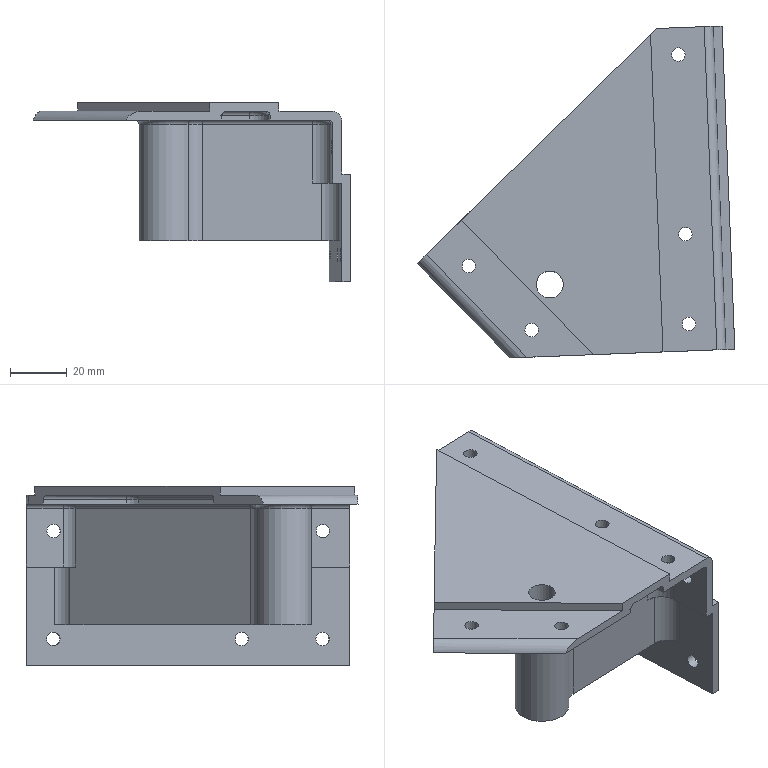Part | NX | features MG0301 nose pivot 24(left) 2 | 1 solid | 85 faces | box 112.244 x 117.328 x 63.5 mm | volume 107943 mm3 | cylinder 40 | plane 33 | torus 12 | commonest cylinder face diameters 12.7 x15 3.15 x10 4.763 x10 9.525 x2 6.35 x1 19.05 x1